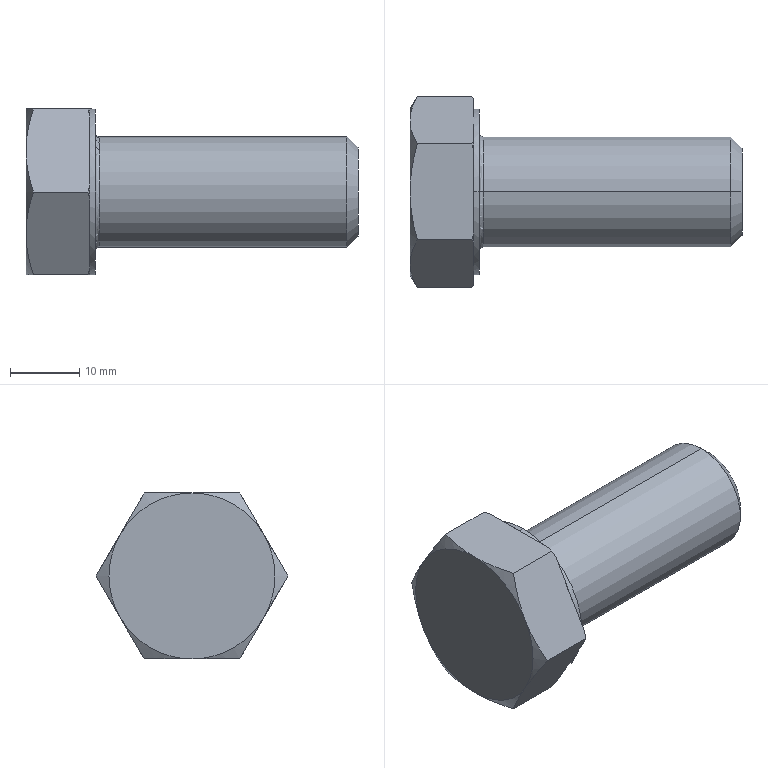Part | SolidWorks | features RevCut 4, Chamfer 1, Extrusion 1, Fillet 1, LPattern 1, Revolution 1 | 1 solid | 35 faces | box 48 x 27.713 x 24 mm | volume 12520 mm3 | plane 15 | cone 14 | cylinder 4 | torus 2 | commonest cylinder face diameters 16 x2 24 x2
STEP:
#1=CARTESIAN_POINT('',(10.6,0.,8.));
#2=VERTEX_POINT('',#1);
#3=CARTESIAN_POINT('',(10.6,0.,-8.));
#4=VERTEX_POINT('',#3);
#5=CARTESIAN_POINT('',(10.6,0.,0.));
#6=DIRECTION('',(1.,0.,0.));
#7=DIRECTION('',(0.,0.,-1.));
#8=AXIS2_PLACEMENT_3D('',#5,#6,#7);
#9=CIRCLE('',#8,8.);
#10=EDGE_CURVE('',#2,#4,#9,.T.);
#11=ORIENTED_EDGE('',*,*,#10,.F.);
#12=CARTESIAN_POINT('',(10.,0.,8.6));
#13=VERTEX_POINT('',#12);
#14=CARTESIAN_POINT('',(10.6,0.,8.6));
#15=DIRECTION('',(0.,1.,0.));
#16=DIRECTION('',(0.,0.,1.));
#17=AXIS2_PLACEMENT_3D('',#14,#15,#16);
#18=CIRCLE('',#17,0.6);
#19=EDGE_CURVE('',#2,#13,#18,.T.);
#20=ORIENTED_EDGE('',*,*,#19,.T.);
#21=CARTESIAN_POINT('',(10.,0.,-8.6));
#22=VERTEX_POINT('',#21);
#23=CARTESIAN_POINT('',(10.,0.,0.));
#24=DIRECTION('',(-1.,0.,0.));
#25=DIRECTION('',(0.,0.,-1.));
#26=AXIS2_PLACEMENT_3D('',#23,#24,#25);
#27=CIRCLE('',#26,8.6);
#28=EDGE_CURVE('',#22,#13,#27,.T.);
#29=ORIENTED_EDGE('',*,*,#28,.F.);
#30=CARTESIAN_POINT('',(10.6,0.,-8.6));
#31=DIRECTION('',(0.,-1.,0.));
#32=DIRECTION('',(0.,0.,-1.));
#33=AXIS2_PLACEMENT_3D('',#30,#31,#32);
#34=CIRCLE('',#33,0.6);
#35=EDGE_CURVE('',#4,#22,#34,.T.);
#36=ORIENTED_EDGE('',*,*,#35,.F.);
#37=EDGE_LOOP('',(#11,#20,#29,#36));
#38=FACE_OUTER_BOUND('',#37,.T.);
#39=CARTESIAN_POINT('',(10.6,0.,0.));
#40=DIRECTION('',(1.,0.,0.));
#41=DIRECTION('',(0.,0.,-1.));
#42=AXIS2_PLACEMENT_3D('',#39,#40,#41);
#43=TOROIDAL_SURFACE('',#42,8.6,0.6);
#44=ADVANCED_FACE('',(#38),#43,.F.);
#45=CARTESIAN_POINT('',(48.,0.,-6.4));
#46=VERTEX_POINT('',#45);
#47=CARTESIAN_POINT('',(48.,0.,6.4));
#48=VERTEX_POINT('',#47);
#49=CARTESIAN_POINT('',(48.,0.,0.));
#50=DIRECTION('',(1.,0.,0.));
#51=DIRECTION('',(0.,0.,1.));
#52=AXIS2_PLACEMENT_3D('',#49,#50,#51);
#53=CIRCLE('',#52,6.4);
#54=EDGE_CURVE('',#46,#48,#53,.T.);
#55=ORIENTED_EDGE('',*,*,#54,.F.);
#56=CARTESIAN_POINT('',(46.4,0.,-8.));
#57=VERTEX_POINT('',#56);
#58=CARTESIAN_POINT('',(46.4,0.,-8.));
#59=DIRECTION('',(-0.7071,0.,-0.7071));
#60=VECTOR('',#59,1000.);
#61=LINE('',#58,#60);
#62=EDGE_CURVE('',#46,#57,#61,.T.);
#63=ORIENTED_EDGE('',*,*,#62,.T.);
#64=CARTESIAN_POINT('',(46.4,0.,8.));
#65=VERTEX_POINT('',#64);
#66=CARTESIAN_POINT('',(46.4,0.,0.));
#67=DIRECTION('',(-1.,0.,0.));
#68=DIRECTION('',(0.,0.,1.));
#69=AXIS2_PLACEMENT_3D('',#66,#67,#68);
#70=CIRCLE('',#69,8.);
#71=EDGE_CURVE('',#65,#57,#70,.T.);
#72=ORIENTED_EDGE('',*,*,#71,.F.);
#73=CARTESIAN_POINT('',(46.4,0.,8.));
#74=DIRECTION('',(-0.7071,0.,0.7071));
#75=VECTOR('',#74,1000.);
#76=LINE('',#73,#75);
#77=EDGE_CURVE('',#48,#65,#76,.T.);
#78=ORIENTED_EDGE('',*,*,#77,.F.);
#79=EDGE_LOOP('',(#55,#63,#72,#78));
#80=FACE_OUTER_BOUND('',#79,.T.);
#81=CARTESIAN_POINT('',(46.4,0.,0.));
#82=DIRECTION('',(-1.,0.,0.));
#83=DIRECTION('',(0.,0.,1.));
#84=AXIS2_PLACEMENT_3D('',#81,#82,#83);
#85=CONICAL_SURFACE('',#84,8.,0.7854);
#86=ADVANCED_FACE('',(#80),#85,.T.);
#87=ORIENTED_EDGE('',*,*,#71,.T.);
#88=CARTESIAN_POINT('',(0.,0.,-8.));
#89=DIRECTION('',(-1.,0.,0.));
#90=VECTOR('',#89,1000.);
#91=LINE('',#88,#90);
#92=EDGE_CURVE('',#57,#4,#91,.T.);
#93=ORIENTED_EDGE('',*,*,#92,.T.);
#94=CARTESIAN_POINT('',(10.6,0.,0.));
#95=DIRECTION('',(1.,0.,0.));
#96=DIRECTION('',(0.,0.,-1.));
#97=AXIS2_PLACEMENT_3D('',#94,#95,#96);
#98=CIRCLE('',#97,8.);
#99=EDGE_CURVE('',#4,#2,#98,.T.);
#100=ORIENTED_EDGE('',*,*,#99,.T.);
#101=CARTESIAN_POINT('',(0.,0.,8.));
#102=DIRECTION('',(-1.,0.,0.));
#103=VECTOR('',#102,1000.);
#104=LINE('',#101,#103);
#105=EDGE_CURVE('',#65,#2,#104,.T.);
#106=ORIENTED_EDGE('',*,*,#105,.F.);
#107=EDGE_LOOP('',(#87,#93,#100,#106));
#108=FACE_OUTER_BOUND('',#107,.T.);
#109=CARTESIAN_POINT('',(0.,0.,0.));
#110=DIRECTION('',(-1.,0.,0.));
#111=DIRECTION('',(0.,0.,1.));
#112=AXIS2_PLACEMENT_3D('',#109,#110,#111);
#113=CYLINDRICAL_SURFACE('',#112,8.);
#114=ADVANCED_FACE('',(#108),#113,.T.);
#115=CARTESIAN_POINT('',(10.,0.,-12.));
#116=VERTEX_POINT('',#115);
#117=CARTESIAN_POINT('',(10.,0.,12.));
#118=VERTEX_POINT('',#117);
#119=CARTESIAN_POINT('',(10.,0.,0.));
#120=DIRECTION('',(1.,0.,0.));
#121=DIRECTION('',(0.,0.,-1.));
#122=AXIS2_PLACEMENT_3D('',#119,#120,#121);
#123=CIRCLE('',#122,12.);
#124=EDGE_CURVE('',#116,#118,#123,.T.);
#125=ORIENTED_EDGE('',*,*,#124,.F.);
#126=CARTESIAN_POINT('',(9.2,0.,-12.));
#127=VERTEX_POINT('',#126);
#128=CARTESIAN_POINT('',(0.,0.,-12.));
#129=DIRECTION('',(-1.,0.,0.));
#130=VECTOR('',#129,1000.);
#131=LINE('',#128,#130);
#132=EDGE_CURVE('',#116,#127,#131,.T.);
#133=ORIENTED_EDGE('',*,*,#132,.T.);
#134=CARTESIAN_POINT('',(9.2,10.392,-6.));
#135=VERTEX_POINT('',#134);
#136=CARTESIAN_POINT('',(9.2,0.,0.));
#137=DIRECTION('',(-1.,0.,0.));
#138=DIRECTION('',(0.,0.,1.));
#139=AXIS2_PLACEMENT_3D('',#136,#137,#138);
#140=CIRCLE('',#139,12.);
#141=EDGE_CURVE('',#135,#127,#140,.T.);
#142=ORIENTED_EDGE('',*,*,#141,.F.);
#143=CARTESIAN_POINT('',(9.2,10.392,6.));
#144=VERTEX_POINT('',#143);
#145=CARTESIAN_POINT('',(9.2,0.,0.));
#146=DIRECTION('',(-1.,0.,0.));
#147=DIRECTION('',(0.,0.,1.));
#148=AXIS2_PLACEMENT_3D('',#145,#146,#147);
#149=CIRCLE('',#148,12.);
#150=EDGE_CURVE('',#144,#135,#149,.T.);
#151=ORIENTED_EDGE('',*,*,#150,.F.);
#152=CARTESIAN_POINT('',(9.2,0.,12.));
#153=VERTEX_POINT('',#152);
#154=CARTESIAN_POINT('',(9.2,0.,0.));
#155=DIRECTION('',(-1.,0.,0.));
#156=DIRECTION('',(0.,0.,1.));
#157=AXIS2_PLACEMENT_3D('',#154,#155,#156);
#158=CIRCLE('',#157,12.);
#159=EDGE_CURVE('',#153,#144,#158,.T.);
#160=ORIENTED_EDGE('',*,*,#159,.F.);
#161=CARTESIAN_POINT('',(0.,0.,12.));
#162=DIRECTION('',(-1.,0.,0.));
#163=VECTOR('',#162,1000.);
#164=LINE('',#161,#163);
#165=EDGE_CURVE('',#118,#153,#164,.T.);
#166=ORIENTED_EDGE('',*,*,#165,.F.);
#167=EDGE_LOOP('',(#125,#133,#142,#151,#160,#166));
#168=FACE_OUTER_BOUND('',#167,.T.);
#169=CARTESIAN_POINT('',(0.,0.,0.));
#170=DIRECTION('',(-1.,0.,0.));
#171=DIRECTION('',(0.,0.,1.));
#172=AXIS2_PLACEMENT_3D('',#169,#170,#171);
#173=CYLINDRICAL_SURFACE('',#172,12.);
#174=ADVANCED_FACE('',(#168),#173,.T.);
#175=CARTESIAN_POINT('',(9.2,7.427,-11.136));
#176=VERTEX_POINT('',#175);
#177=CARTESIAN_POINT('',(9.2,6.928,-12.));
#178=DIRECTION('',(0.,0.5,0.866));
#179=VECTOR('',#178,1000.);
#180=LINE('',#177,#179);
#181=EDGE_CURVE('',#176,#135,#180,.T.);
#182=ORIENTED_EDGE('',*,*,#181,.F.);
#183=CARTESIAN_POINT('',(8.928,6.928,-12.));
#184=VERTEX_POINT('',#183);
#185=CARTESIAN_POINT('',(8.928,6.928,-12.));
#186=CARTESIAN_POINT('',(9.024,7.094,-11.713));
#187=CARTESIAN_POINT('',(9.115,7.26,-11.425));
#188=CARTESIAN_POINT('',(9.2,7.427,-11.136));
#189=B_SPLINE_CURVE_WITH_KNOTS('',3,(#185,#186,#187,#188),.UNSPECIFIED.,.F.,.F.,(4,4),(0.000000238,0.001026),.UNSPECIFIED.);
#190=EDGE_CURVE('',#184,#176,#189,.T.);
#191=ORIENTED_EDGE('',*,*,#190,.F.);
#192=CARTESIAN_POINT('',(1.072,6.928,-12.));
#193=VERTEX_POINT('',#192);
#194=CARTESIAN_POINT('',(10.,6.928,-12.));
#195=DIRECTION('',(-1.,0.,0.));
#196=VECTOR('',#195,1000.);
#197=LINE('',#194,#196);
#198=EDGE_CURVE('',#184,#193,#197,.T.);
#199=ORIENTED_EDGE('',*,*,#198,.T.);
#200=CARTESIAN_POINT('',(0.,10.392,-6.));
#201=VERTEX_POINT('',#200);
#202=CARTESIAN_POINT('',(0.,10.392,-6.));
#203=CARTESIAN_POINT('',(0.,10.098,-6.509));
#204=CARTESIAN_POINT('',(0.02533,9.803,-7.021));
#205=CARTESIAN_POINT('',(0.1234,9.219,-8.033));
#206=CARTESIAN_POINT('',(0.196,8.929,-8.535));
#207=CARTESIAN_POINT('',(0.476,8.063,-10.034));
#208=CARTESIAN_POINT('',(0.7454,7.493,-11.021));
#209=CARTESIAN_POINT('',(1.072,6.928,-12.));
#210=B_SPLINE_CURVE_WITH_KNOTS('',3,(#202,#203,#204,#205,#206,#207,#208,#209),.UNSPECIFIED.,.F.,.F.,(4,2,2,4),(0.00701,0.008756,0.0105,0.01399),.UNSPECIFIED.);
#211=EDGE_CURVE('',#201,#193,#210,.T.);
#212=ORIENTED_EDGE('',*,*,#211,.F.);
#213=CARTESIAN_POINT('',(1.072,13.856,0.));
#214=VERTEX_POINT('',#213);
#215=CARTESIAN_POINT('',(1.072,13.856,0.));
#216=CARTESIAN_POINT('',(0.7446,13.29,-0.9815));
#217=CARTESIAN_POINT('',(0.4751,12.719,-1.97));
#218=CARTESIAN_POINT('',(0.1021,11.565,-3.968));
#219=CARTESIAN_POINT('',(0.,10.982,-4.978));
#220=CARTESIAN_POINT('',(0.,10.392,-6.));
#221=B_SPLINE_CURVE_WITH_KNOTS('',3,(#215,#216,#217,#218,#219,#220),.UNSPECIFIED.,.F.,.F.,(4,2,4),(0.000000238,0.003505,0.00701),.UNSPECIFIED.);
#222=EDGE_CURVE('',#214,#201,#221,.T.);
#223=ORIENTED_EDGE('',*,*,#222,.F.);
#224=CARTESIAN_POINT('',(8.928,13.856,0.));
#225=VERTEX_POINT('',#224);
#226=CARTESIAN_POINT('',(10.,13.856,0.));
#227=DIRECTION('',(-1.,0.,0.));
#228=VECTOR('',#227,1000.);
#229=LINE('',#226,#228);
#230=EDGE_CURVE('',#225,#214,#229,.T.);
#231=ORIENTED_EDGE('',*,*,#230,.F.);
#232=CARTESIAN_POINT('',(9.2,13.358,-0.8637));
#233=VERTEX_POINT('',#232);
#234=CARTESIAN_POINT('',(9.2,13.358,-0.8637));
#235=CARTESIAN_POINT('',(9.115,13.524,-0.575));
#236=CARTESIAN_POINT('',(9.024,13.691,-0.2872));
#237=CARTESIAN_POINT('',(8.928,13.856,0.));
#238=B_SPLINE_CURVE_WITH_KNOTS('',3,(#234,#235,#236,#237),.UNSPECIFIED.,.F.,.F.,(4,4),(0.01297,0.01399),.UNSPECIFIED.);
#239=EDGE_CURVE('',#233,#225,#238,.T.);
#240=ORIENTED_EDGE('',*,*,#239,.F.);
#241=CARTESIAN_POINT('',(9.2,6.928,-12.));
#242=DIRECTION('',(0.,0.5,0.866));
#243=VECTOR('',#242,1000.);
#244=LINE('',#241,#243);
#245=EDGE_CURVE('',#135,#233,#244,.T.);
#246=ORIENTED_EDGE('',*,*,#245,.F.);
#247=EDGE_LOOP('',(#182,#191,#199,#212,#223,#231,#240,#246));
#248=FACE_OUTER_BOUND('',#247,.T.);
#249=CARTESIAN_POINT('',(10.,6.928,-12.));
#250=DIRECTION('',(0.,-0.866,0.5));
#251=DIRECTION('',(0.,-0.5,-0.866));
#252=AXIS2_PLACEMENT_3D('',#249,#250,#251);
#253=PLANE('',#252);
#254=ADVANCED_FACE('',(#248),#253,.F.);
#255=CARTESIAN_POINT('',(9.2,13.358,0.8637));
#256=VERTEX_POINT('',#255);
#257=CARTESIAN_POINT('',(9.2,13.856,0.));
#258=DIRECTION('',(0.,-0.5,0.866));
#259=VECTOR('',#258,1000.);
#260=LINE('',#257,#259);
#261=EDGE_CURVE('',#256,#144,#260,.T.);
#262=ORIENTED_EDGE('',*,*,#261,.F.);
#263=CARTESIAN_POINT('',(8.928,13.856,0.));
#264=CARTESIAN_POINT('',(9.024,13.691,0.2873));
#265=CARTESIAN_POINT('',(9.115,13.524,0.5751));
#266=CARTESIAN_POINT('',(9.2,13.358,0.8637));
#267=B_SPLINE_CURVE_WITH_KNOTS('',3,(#263,#264,#265,#266),.UNSPECIFIED.,.F.,.F.,(4,4),(0.000000238,0.001026),.UNSPECIFIED.);
#268=EDGE_CURVE('',#225,#256,#267,.T.);
#269=ORIENTED_EDGE('',*,*,#268,.F.);
#270=ORIENTED_EDGE('',*,*,#230,.T.);
#271=CARTESIAN_POINT('',(0.,10.392,6.));
#272=VERTEX_POINT('',#271);
#273=CARTESIAN_POINT('',(0.,10.392,6.));
#274=CARTESIAN_POINT('',(0.,10.686,5.491));
#275=CARTESIAN_POINT('',(0.02533,10.982,4.979));
#276=CARTESIAN_POINT('',(0.1234,11.566,3.967));
#277=CARTESIAN_POINT('',(0.196,11.856,3.465));
#278=CARTESIAN_POINT('',(0.476,12.721,1.966));
#279=CARTESIAN_POINT('',(0.7454,13.291,0.9791));
#280=CARTESIAN_POINT('',(1.072,13.856,0.));
#281=B_SPLINE_CURVE_WITH_KNOTS('',3,(#273,#274,#275,#276,#277,#278,#279,#280),.UNSPECIFIED.,.F.,.F.,(4,2,2,4),(0.00701,0.008756,0.0105,0.01399),.UNSPECIFIED.);
#282=EDGE_CURVE('',#272,#214,#281,.T.);
#283=ORIENTED_EDGE('',*,*,#282,.F.);
#284=CARTESIAN_POINT('',(1.072,6.928,12.));
#285=VERTEX_POINT('',#284);
#286=CARTESIAN_POINT('',(1.072,6.928,12.));
#287=CARTESIAN_POINT('',(0.7446,7.495,11.018));
#288=CARTESIAN_POINT('',(0.4751,8.066,10.03));
#289=CARTESIAN_POINT('',(0.1021,9.219,8.032));
#290=CARTESIAN_POINT('',(0.,9.802,7.022));
#291=CARTESIAN_POINT('',(0.,10.392,6.));
#292=B_SPLINE_CURVE_WITH_KNOTS('',3,(#286,#287,#288,#289,#290,#291),.UNSPECIFIED.,.F.,.F.,(4,2,4),(0.000000238,0.003505,0.00701),.UNSPECIFIED.);
#293=EDGE_CURVE('',#285,#272,#292,.T.);
#294=ORIENTED_EDGE('',*,*,#293,.F.);
#295=CARTESIAN_POINT('',(8.928,6.928,12.));
#296=VERTEX_POINT('',#295);
#297=CARTESIAN_POINT('',(10.,6.928,12.));
#298=DIRECTION('',(-1.,0.,0.));
#299=VECTOR('',#298,1000.);
#300=LINE('',#297,#299);
#301=EDGE_CURVE('',#296,#285,#300,.T.);
#302=ORIENTED_EDGE('',*,*,#301,.F.);
#303=CARTESIAN_POINT('',(9.2,7.427,11.136));
#304=VERTEX_POINT('',#303);
#305=CARTESIAN_POINT('',(9.2,7.427,11.136));
#306=CARTESIAN_POINT('',(9.115,7.26,11.425));
#307=CARTESIAN_POINT('',(9.024,7.094,11.713));
#308=CARTESIAN_POINT('',(8.928,6.928,12.));
#309=B_SPLINE_CURVE_WITH_KNOTS('',3,(#305,#306,#307,#308),.UNSPECIFIED.,.F.,.F.,(4,4),(0.01297,0.01399),.UNSPECIFIED.);
#310=EDGE_CURVE('',#304,#296,#309,.T.);
#311=ORIENTED_EDGE('',*,*,#310,.F.);
#312=CARTESIAN_POINT('',(9.2,13.856,0.));
#313=DIRECTION('',(0.,-0.5,0.866));
#314=VECTOR('',#313,1000.);
#315=LINE('',#312,#314);
#316=EDGE_CURVE('',#144,#304,#315,.T.);
#317=ORIENTED_EDGE('',*,*,#316,.F.);
#318=EDGE_LOOP('',(#262,#269,#270,#283,#294,#302,#311,#317));
#319=FACE_OUTER_BOUND('',#318,.T.);
#320=CARTESIAN_POINT('',(10.,13.856,0.));
#321=DIRECTION('',(0.,-0.866,-0.5));
#322=DIRECTION('',(0.,0.5,-0.866));
#323=AXIS2_PLACEMENT_3D('',#320,#321,#322);
#324=PLANE('',#323);
#325=ADVANCED_FACE('',(#319),#324,.F.);
#326=CARTESIAN_POINT('',(9.2,5.931,12.));
#327=VERTEX_POINT('',#326);
#328=CARTESIAN_POINT('',(9.2,6.928,12.));
#329=DIRECTION('',(0.,-1.,0.));
#330=VECTOR('',#329,1000.);
#331=LINE('',#328,#330);
#332=EDGE_CURVE('',#327,#153,#331,.T.);
#333=ORIENTED_EDGE('',*,*,#332,.F.);
#334=CARTESIAN_POINT('',(8.928,6.928,12.));
#335=CARTESIAN_POINT('',(9.024,6.597,12.));
#336=CARTESIAN_POINT('',(9.115,6.265,12.));
#337=CARTESIAN_POINT('',(9.2,5.931,12.));
#338=B_SPLINE_CURVE_WITH_KNOTS('',3,(#334,#335,#336,#337),.UNSPECIFIED.,.F.,.F.,(4,4),(0.03236,0.0334),.UNSPECIFIED.);
#339=EDGE_CURVE('',#296,#327,#338,.T.);
#340=ORIENTED_EDGE('',*,*,#339,.F.);
#341=ORIENTED_EDGE('',*,*,#301,.T.);
#342=CARTESIAN_POINT('',(0.,0.,12.));
#343=VERTEX_POINT('',#342);
#344=CARTESIAN_POINT('',(0.,0.,12.));
#345=CARTESIAN_POINT('',(0.,0.5865,12.));
#346=CARTESIAN_POINT('',(0.02506,1.176,12.));
#347=CARTESIAN_POINT('',(0.1242,2.355,12.));
#348=CARTESIAN_POINT('',(0.1975,2.939,12.));
#349=CARTESIAN_POINT('',(0.4791,4.673,12.));
#350=CARTESIAN_POINT('',(0.7483,5.808,12.));
#351=CARTESIAN_POINT('',(1.072,6.928,12.));
#352=B_SPLINE_CURVE_WITH_KNOTS('',3,(#344,#345,#346,#347,#348,#349,#350,#351),.UNSPECIFIED.,.F.,.F.,(4,2,2,4),(0.01982,0.02158,0.02333,0.02684),.UNSPECIFIED.);
#353=EDGE_CURVE('',#343,#285,#352,.T.);
#354=ORIENTED_EDGE('',*,*,#353,.F.);
#355=CARTESIAN_POINT('',(1.072,-6.928,12.));
#356=VERTEX_POINT('',#355);
#357=CARTESIAN_POINT('',(1.072,-6.928,12.));
#358=CARTESIAN_POINT('',(0.7461,-5.8,12.));
#359=CARTESIAN_POINT('',(0.4736,-4.647,12.));
#360=CARTESIAN_POINT('',(0.1008,-2.335,12.));
#361=CARTESIAN_POINT('',(0.,-1.172,12.));
#362=CARTESIAN_POINT('',(0.,0.,12.));
#363=B_SPLINE_CURVE_WITH_KNOTS('',3,(#357,#358,#359,#360,#361,#362),.UNSPECIFIED.,.F.,.F.,(4,2,4),(0.01281,0.01632,0.01982),.UNSPECIFIED.);
#364=EDGE_CURVE('',#356,#343,#363,.T.);
#365=ORIENTED_EDGE('',*,*,#364,.F.);
#366=CARTESIAN_POINT('',(8.928,-6.928,12.));
#367=VERTEX_POINT('',#366);
#368=CARTESIAN_POINT('',(10.,-6.928,12.));
#369=DIRECTION('',(-1.,0.,0.));
#370=VECTOR('',#369,1000.);
#371=LINE('',#368,#370);
#372=EDGE_CURVE('',#367,#356,#371,.T.);
#373=ORIENTED_EDGE('',*,*,#372,.F.);
#374=CARTESIAN_POINT('',(9.2,-5.931,12.));
#375=VERTEX_POINT('',#374);
#376=CARTESIAN_POINT('',(9.2,-5.931,12.));
#377=CARTESIAN_POINT('',(9.114,-6.265,12.));
#378=CARTESIAN_POINT('',(9.024,-6.598,12.));
#379=CARTESIAN_POINT('',(8.928,-6.928,12.));
#380=B_SPLINE_CURVE_WITH_KNOTS('',3,(#376,#377,#378,#379),.UNSPECIFIED.,.F.,.F.,(4,4),(0.04537,0.0464),.UNSPECIFIED.);
#381=EDGE_CURVE('',#375,#367,#380,.T.);
#382=ORIENTED_EDGE('',*,*,#381,.F.);
#383=CARTESIAN_POINT('',(9.2,6.928,12.));
#384=DIRECTION('',(0.,-1.,0.));
#385=VECTOR('',#384,1000.);
#386=LINE('',#383,#385);
#387=EDGE_CURVE('',#153,#375,#386,.T.);
#388=ORIENTED_EDGE('',*,*,#387,.F.);
#389=EDGE_LOOP('',(#333,#340,#341,#354,#365,#373,#382,#388));
#390=FACE_OUTER_BOUND('',#389,.T.);
#391=CARTESIAN_POINT('',(10.,6.928,12.));
#392=DIRECTION('',(0.,0.,-1.));
#393=DIRECTION('',(-1.,0.,0.));
#394=AXIS2_PLACEMENT_3D('',#391,#392,#393);
#395=PLANE('',#394);
#396=ADVANCED_FACE('',(#390),#395,.F.);
#397=CARTESIAN_POINT('',(9.2,-7.427,11.136));
#398=VERTEX_POINT('',#397);
#399=CARTESIAN_POINT('',(9.2,-10.392,6.));
#400=VERTEX_POINT('',#399);
#401=CARTESIAN_POINT('',(9.2,-13.856,0.));
#402=DIRECTION('',(0.,-0.5,-0.866));
#403=VECTOR('',#402,1000.);
#404=LINE('',#401,#403);
#405=EDGE_CURVE('',#398,#400,#404,.T.);
#406=ORIENTED_EDGE('',*,*,#405,.F.);
#407=CARTESIAN_POINT('',(8.928,-6.928,12.));
#408=CARTESIAN_POINT('',(9.024,-7.094,11.713));
#409=CARTESIAN_POINT('',(9.115,-7.26,11.425));
#410=CARTESIAN_POINT('',(9.2,-7.427,11.136));
#411=B_SPLINE_CURVE_WITH_KNOTS('',3,(#407,#408,#409,#410),.UNSPECIFIED.,.F.,.F.,(4,4),(0.000000238,0.001026),.UNSPECIFIED.);
#412=EDGE_CURVE('',#367,#398,#411,.T.);
#413=ORIENTED_EDGE('',*,*,#412,.F.);
#414=ORIENTED_EDGE('',*,*,#372,.T.);
#415=CARTESIAN_POINT('',(0.,-10.392,6.));
#416=VERTEX_POINT('',#415);
#417=CARTESIAN_POINT('',(0.,-10.392,6.));
#418=CARTESIAN_POINT('',(0.,-10.098,6.509));
#419=CARTESIAN_POINT('',(0.02533,-9.803,7.021));
#420=CARTESIAN_POINT('',(0.1234,-9.219,8.033));
#421=CARTESIAN_POINT('',(0.196,-8.929,8.535));
#422=CARTESIAN_POINT('',(0.476,-8.063,10.034));
#423=CARTESIAN_POINT('',(0.7454,-7.493,11.021));
#424=CARTESIAN_POINT('',(1.072,-6.928,12.));
#425=B_SPLINE_CURVE_WITH_KNOTS('',3,(#417,#418,#419,#420,#421,#422,#423,#424),.UNSPECIFIED.,.F.,.F.,(4,2,2,4),(0.00701,0.008756,0.0105,0.01399),.UNSPECIFIED.);
#426=EDGE_CURVE('',#416,#356,#425,.T.);
#427=ORIENTED_EDGE('',*,*,#426,.F.);
#428=CARTESIAN_POINT('',(1.072,-13.856,0.));
#429=VERTEX_POINT('',#428);
#430=CARTESIAN_POINT('',(1.072,-13.856,0.));
#431=CARTESIAN_POINT('',(0.7446,-13.29,0.9815));
#432=CARTESIAN_POINT('',(0.4751,-12.719,1.97));
#433=CARTESIAN_POINT('',(0.1021,-11.565,3.968));
#434=CARTESIAN_POINT('',(0.,-10.982,4.978));
#435=CARTESIAN_POINT('',(0.,-10.392,6.));
#436=B_SPLINE_CURVE_WITH_KNOTS('',3,(#430,#431,#432,#433,#434,#435),.UNSPECIFIED.,.F.,.F.,(4,2,4),(0.000000238,0.003505,0.00701),.UNSPECIFIED.);
#437=EDGE_CURVE('',#429,#416,#436,.T.);
#438=ORIENTED_EDGE('',*,*,#437,.F.);
#439=CARTESIAN_POINT('',(8.928,-13.856,0.));
#440=VERTEX_POINT('',#439);
#441=CARTESIAN_POINT('',(10.,-13.856,0.));
#442=DIRECTION('',(-1.,0.,0.));
#443=VECTOR('',#442,1000.);
#444=LINE('',#441,#443);
#445=EDGE_CURVE('',#440,#429,#444,.T.);
#446=ORIENTED_EDGE('',*,*,#445,.F.);
#447=CARTESIAN_POINT('',(9.2,-13.358,0.8637));
#448=VERTEX_POINT('',#447);
#449=CARTESIAN_POINT('',(9.2,-13.358,0.8637));
#450=CARTESIAN_POINT('',(9.115,-13.524,0.575));
#451=CARTESIAN_POINT('',(9.024,-13.691,0.2872));
#452=CARTESIAN_POINT('',(8.928,-13.856,0.));
#453=B_SPLINE_CURVE_WITH_KNOTS('',3,(#449,#450,#451,#452),.UNSPECIFIED.,.F.,.F.,(4,4),(0.01297,0.01399),.UNSPECIFIED.);
#454=EDGE_CURVE('',#448,#440,#453,.T.);
#455=ORIENTED_EDGE('',*,*,#454,.F.);
#456=CARTESIAN_POINT('',(9.2,-13.856,0.));
#457=DIRECTION('',(0.,-0.5,-0.866));
#458=VECTOR('',#457,1000.);
#459=LINE('',#456,#458);
#460=EDGE_CURVE('',#400,#448,#459,.T.);
#461=ORIENTED_EDGE('',*,*,#460,.F.);
#462=EDGE_LOOP('',(#406,#413,#414,#427,#438,#446,#455,#461));
#463=FACE_OUTER_BOUND('',#462,.T.);
#464=CARTESIAN_POINT('',(10.,-13.856,0.));
#465=DIRECTION('',(0.,0.866,-0.5));
#466=DIRECTION('',(0.,0.5,0.866));
#467=AXIS2_PLACEMENT_3D('',#464,#465,#466);
#468=PLANE('',#467);
#469=ADVANCED_FACE('',(#463),#468,.F.);
#470=CARTESIAN_POINT('',(9.2,-13.358,-0.8637));
#471=VERTEX_POINT('',#470);
#472=CARTESIAN_POINT('',(9.2,-10.392,-6.));
#473=VERTEX_POINT('',#472);
#474=CARTESIAN_POINT('',(9.2,-6.928,-12.));
#475=DIRECTION('',(0.,0.5,-0.866));
#476=VECTOR('',#475,1000.);
#477=LINE('',#474,#476);
#478=EDGE_CURVE('',#471,#473,#477,.T.);
#479=ORIENTED_EDGE('',*,*,#478,.F.);
#480=CARTESIAN_POINT('',(8.928,-13.856,0.));
#481=CARTESIAN_POINT('',(9.024,-13.691,-0.2873));
#482=CARTESIAN_POINT('',(9.115,-13.524,-0.5751));
#483=CARTESIAN_POINT('',(9.2,-13.358,-0.8637));
#484=B_SPLINE_CURVE_WITH_KNOTS('',3,(#480,#481,#482,#483),.UNSPECIFIED.,.F.,.F.,(4,4),(0.000000238,0.001026),.UNSPECIFIED.);
#485=EDGE_CURVE('',#440,#471,#484,.T.);
#486=ORIENTED_EDGE('',*,*,#485,.F.);
#487=ORIENTED_EDGE('',*,*,#445,.T.);
#488=CARTESIAN_POINT('',(0.,-10.392,-6.));
#489=VERTEX_POINT('',#488);
#490=CARTESIAN_POINT('',(0.,-10.392,-6.));
#491=CARTESIAN_POINT('',(0.,-10.686,-5.491));
#492=CARTESIAN_POINT('',(0.02533,-10.982,-4.979));
#493=CARTESIAN_POINT('',(0.1234,-11.566,-3.967));
#494=CARTESIAN_POINT('',(0.196,-11.856,-3.465));
#495=CARTESIAN_POINT('',(0.476,-12.721,-1.966));
#496=CARTESIAN_POINT('',(0.7454,-13.291,-0.9791));
#497=CARTESIAN_POINT('',(1.072,-13.856,0.));
#498=B_SPLINE_CURVE_WITH_KNOTS('',3,(#490,#491,#492,#493,#494,#495,#496,#497),.UNSPECIFIED.,.F.,.F.,(4,2,2,4),(0.00701,0.008756,0.0105,0.01399),.UNSPECIFIED.);
#499=EDGE_CURVE('',#489,#429,#498,.T.);
#500=ORIENTED_EDGE('',*,*,#499,.F.);
#501=CARTESIAN_POINT('',(1.072,-6.928,-12.));
#502=VERTEX_POINT('',#501);
#503=CARTESIAN_POINT('',(1.072,-6.928,-12.));
#504=CARTESIAN_POINT('',(0.7446,-7.495,-11.018));
#505=CARTESIAN_POINT('',(0.4751,-8.066,-10.03));
#506=CARTESIAN_POINT('',(0.1021,-9.219,-8.032));
#507=CARTESIAN_POINT('',(0.,-9.802,-7.022));
#508=CARTESIAN_POINT('',(0.,-10.392,-6.));
#509=B_SPLINE_CURVE_WITH_KNOTS('',3,(#503,#504,#505,#506,#507,#508),.UNSPECIFIED.,.F.,.F.,(4,2,4),(0.000000238,0.003505,0.00701),.UNSPECIFIED.);
#510=EDGE_CURVE('',#502,#489,#509,.T.);
#511=ORIENTED_EDGE('',*,*,#510,.F.);
#512=CARTESIAN_POINT('',(8.928,-6.928,-12.));
#513=VERTEX_POINT('',#512);
#514=CARTESIAN_POINT('',(10.,-6.928,-12.));
#515=DIRECTION('',(-1.,0.,0.));
#516=VECTOR('',#515,1000.);
#517=LINE('',#514,#516);
#518=EDGE_CURVE('',#513,#502,#517,.T.);
#519=ORIENTED_EDGE('',*,*,#518,.F.);
#520=CARTESIAN_POINT('',(9.2,-7.427,-11.136));
#521=VERTEX_POINT('',#520);
#522=CARTESIAN_POINT('',(9.2,-7.427,-11.136));
#523=CARTESIAN_POINT('',(9.115,-7.26,-11.425));
#524=CARTESIAN_POINT('',(9.024,-7.094,-11.713));
#525=CARTESIAN_POINT('',(8.928,-6.928,-12.));
#526=B_SPLINE_CURVE_WITH_KNOTS('',3,(#522,#523,#524,#525),.UNSPECIFIED.,.F.,.F.,(4,4),(0.01297,0.01399),.UNSPECIFIED.);
#527=EDGE_CURVE('',#521,#513,#526,.T.);
#528=ORIENTED_EDGE('',*,*,#527,.F.);
#529=CARTESIAN_POINT('',(9.2,-6.928,-12.));
#530=DIRECTION('',(0.,0.5,-0.866));
#531=VECTOR('',#530,1000.);
#532=LINE('',#529,#531);
#533=EDGE_CURVE('',#473,#521,#532,.T.);
#534=ORIENTED_EDGE('',*,*,#533,.F.);
#535=EDGE_LOOP('',(#479,#486,#487,#500,#511,#519,#528,#534));
#536=FACE_OUTER_BOUND('',#535,.T.);
#537=CARTESIAN_POINT('',(10.,-6.928,-12.));
#538=DIRECTION('',(0.,0.866,0.5));
#539=DIRECTION('',(0.,-0.5,0.866));
#540=AXIS2_PLACEMENT_3D('',#537,#538,#539);
#541=PLANE('',#540);
#542=ADVANCED_FACE('',(#536),#541,.F.);
#543=CARTESIAN_POINT('',(9.2,-5.931,-12.));
#544=VERTEX_POINT('',#543);
#545=CARTESIAN_POINT('',(9.2,6.928,-12.));
#546=DIRECTION('',(0.,1.,0.));
#547=VECTOR('',#546,1000.);
#548=LINE('',#545,#547);
#549=EDGE_CURVE('',#544,#127,#548,.T.);
#550=ORIENTED_EDGE('',*,*,#549,.F.);
#551=CARTESIAN_POINT('',(8.928,-6.928,-12.));
#552=CARTESIAN_POINT('',(9.024,-6.598,-12.));
#553=CARTESIAN_POINT('',(9.114,-6.265,-12.));
#554=CARTESIAN_POINT('',(9.2,-5.931,-12.));
#555=B_SPLINE_CURVE_WITH_KNOTS('',3,(#551,#552,#553,#554),.UNSPECIFIED.,.F.,.F.,(4,4),(0.01281,0.01384),.UNSPECIFIED.);
#556=EDGE_CURVE('',#513,#544,#555,.T.);
#557=ORIENTED_EDGE('',*,*,#556,.F.);
#558=ORIENTED_EDGE('',*,*,#518,.T.);
#559=CARTESIAN_POINT('',(0.,0.,-12.));
#560=VERTEX_POINT('',#559);
#561=CARTESIAN_POINT('',(0.,0.,-12.));
#562=CARTESIAN_POINT('',(0.,-1.172,-12.));
#563=CARTESIAN_POINT('',(0.1008,-2.335,-12.));
#564=CARTESIAN_POINT('',(0.4736,-4.647,-12.));
#565=CARTESIAN_POINT('',(0.7461,-5.8,-12.));
#566=CARTESIAN_POINT('',(1.072,-6.928,-12.));
#567=B_SPLINE_CURVE_WITH_KNOTS('',3,(#561,#562,#563,#564,#565,#566),.UNSPECIFIED.,.F.,.F.,(4,2,4),(0.03938,0.04289,0.0464),.UNSPECIFIED.);
#568=EDGE_CURVE('',#560,#502,#567,.T.);
#569=ORIENTED_EDGE('',*,*,#568,.F.);
#570=CARTESIAN_POINT('',(1.072,6.928,-12.));
#571=CARTESIAN_POINT('',(0.7483,5.808,-12.));
#572=CARTESIAN_POINT('',(0.4791,4.673,-12.));
#573=CARTESIAN_POINT('',(0.1975,2.939,-12.));
#574=CARTESIAN_POINT('',(0.1242,2.355,-12.));
#575=CARTESIAN_POINT('',(0.02506,1.176,-12.));
#576=CARTESIAN_POINT('',(0.,0.5865,-12.));
#577=CARTESIAN_POINT('',(0.,0.,-12.));
#578=B_SPLINE_CURVE_WITH_KNOTS('',3,(#570,#571,#572,#573,#574,#575,#576,#577),.UNSPECIFIED.,.F.,.F.,(4,2,2,4),(0.03236,0.03587,0.03763,0.03938),.UNSPECIFIED.);
#579=EDGE_CURVE('',#193,#560,#578,.T.);
#580=ORIENTED_EDGE('',*,*,#579,.F.);
#581=ORIENTED_EDGE('',*,*,#198,.F.);
#582=CARTESIAN_POINT('',(9.2,5.931,-12.));
#583=VERTEX_POINT('',#582);
#584=CARTESIAN_POINT('',(9.2,5.931,-12.));
#585=CARTESIAN_POINT('',(9.115,6.265,-12.));
#586=CARTESIAN_POINT('',(9.024,6.597,-12.));
#587=CARTESIAN_POINT('',(8.928,6.928,-12.));
#588=B_SPLINE_CURVE_WITH_KNOTS('',3,(#584,#585,#586,#587),.UNSPECIFIED.,.F.,.F.,(4,4),(0.0258,0.02684),.UNSPECIFIED.);
#589=EDGE_CURVE('',#583,#184,#588,.T.);
#590=ORIENTED_EDGE('',*,*,#589,.F.);
#591=CARTESIAN_POINT('',(9.2,6.928,-12.));
#592=DIRECTION('',(0.,1.,0.));
#593=VECTOR('',#592,1000.);
#594=LINE('',#591,#593);
#595=EDGE_CURVE('',#127,#583,#594,.T.);
#596=ORIENTED_EDGE('',*,*,#595,.F.);
#597=EDGE_LOOP('',(#550,#557,#558,#569,#580,#581,#590,#596));
#598=FACE_OUTER_BOUND('',#597,.T.);
#599=CARTESIAN_POINT('',(10.,6.928,-12.));
#600=DIRECTION('',(0.,0.,1.));
#601=DIRECTION('',(0.,-1.,0.));
#602=AXIS2_PLACEMENT_3D('',#599,#600,#601);
#603=PLANE('',#602);
#604=ADVANCED_FACE('',(#598),#603,.F.);
#605=ORIENTED_EDGE('',*,*,#556,.T.);
#606=CARTESIAN_POINT('',(9.2,0.,0.));
#607=DIRECTION('',(-1.,0.,0.));
#608=DIRECTION('',(0.,0.,-1.));
#609=AXIS2_PLACEMENT_3D('',#606,#607,#608);
#610=CIRCLE('',#609,13.386);
#611=EDGE_CURVE('',#544,#521,#610,.T.);
#612=ORIENTED_EDGE('',*,*,#611,.T.);
#613=ORIENTED_EDGE('',*,*,#527,.T.);
#614=EDGE_LOOP('',(#605,#612,#613));
#615=FACE_OUTER_BOUND('',#614,.T.);
#616=CARTESIAN_POINT('',(6.041,0.,0.));
#617=DIRECTION('',(-1.,0.,0.));
#618=DIRECTION('',(0.,0.,1.));
#619=AXIS2_PLACEMENT_3D('',#616,#617,#618);
#620=CONICAL_SURFACE('',#619,18.856,1.047);
#621=ADVANCED_FACE('',(#615),#620,.T.);
#622=ORIENTED_EDGE('',*,*,#485,.T.);
#623=CARTESIAN_POINT('',(9.2,0.,0.));
#624=DIRECTION('',(-1.,0.,0.));
#625=DIRECTION('',(0.,0.,-1.));
#626=AXIS2_PLACEMENT_3D('',#623,#624,#625);
#627=CIRCLE('',#626,13.386);
#628=EDGE_CURVE('',#471,#448,#627,.T.);
#629=ORIENTED_EDGE('',*,*,#628,.T.);
#630=ORIENTED_EDGE('',*,*,#454,.T.);
#631=EDGE_LOOP('',(#622,#629,#630));
#632=FACE_OUTER_BOUND('',#631,.T.);
#633=CARTESIAN_POINT('',(6.041,0.,0.));
#634=DIRECTION('',(-1.,0.,0.));
#635=DIRECTION('',(0.,0.,1.));
#636=AXIS2_PLACEMENT_3D('',#633,#634,#635);
#637=CONICAL_SURFACE('',#636,18.856,1.047);
#638=ADVANCED_FACE('',(#632),#637,.T.);
#639=ORIENTED_EDGE('',*,*,#412,.T.);
#640=CARTESIAN_POINT('',(9.2,0.,0.));
#641=DIRECTION('',(-1.,0.,0.));
#642=DIRECTION('',(0.,0.,-1.));
#643=AXIS2_PLACEMENT_3D('',#640,#641,#642);
#644=CIRCLE('',#643,13.386);
#645=EDGE_CURVE('',#398,#375,#644,.T.);
#646=ORIENTED_EDGE('',*,*,#645,.T.);
#647=ORIENTED_EDGE('',*,*,#381,.T.);
#648=EDGE_LOOP('',(#639,#646,#647));
#649=FACE_OUTER_BOUND('',#648,.T.);
#650=CARTESIAN_POINT('',(6.041,0.,0.));
#651=DIRECTION('',(-1.,0.,0.));
#652=DIRECTION('',(0.,0.,1.));
#653=AXIS2_PLACEMENT_3D('',#650,#651,#652);
#654=CONICAL_SURFACE('',#653,18.856,1.047);
#655=ADVANCED_FACE('',(#649),#654,.T.);
#656=ORIENTED_EDGE('',*,*,#339,.T.);
#657=CARTESIAN_POINT('',(9.2,0.,0.));
#658=DIRECTION('',(-1.,0.,0.));
#659=DIRECTION('',(0.,0.,-1.));
#660=AXIS2_PLACEMENT_3D('',#657,#658,#659);
#661=CIRCLE('',#660,13.386);
#662=EDGE_CURVE('',#327,#304,#661,.T.);
#663=ORIENTED_EDGE('',*,*,#662,.T.);
#664=ORIENTED_EDGE('',*,*,#310,.T.);
#665=EDGE_LOOP('',(#656,#663,#664));
#666=FACE_OUTER_BOUND('',#665,.T.);
#667=CARTESIAN_POINT('',(6.041,0.,0.));
#668=DIRECTION('',(-1.,0.,0.));
#669=DIRECTION('',(0.,0.,1.));
#670=AXIS2_PLACEMENT_3D('',#667,#668,#669);
#671=CONICAL_SURFACE('',#670,18.856,1.047);
#672=ADVANCED_FACE('',(#666),#671,.T.);
#673=ORIENTED_EDGE('',*,*,#268,.T.);
#674=CARTESIAN_POINT('',(9.2,0.,0.));
#675=DIRECTION('',(-1.,0.,0.));
#676=DIRECTION('',(0.,0.,-1.));
#677=AXIS2_PLACEMENT_3D('',#674,#675,#676);
#678=CIRCLE('',#677,13.386);
#679=EDGE_CURVE('',#256,#233,#678,.T.);
#680=ORIENTED_EDGE('',*,*,#679,.T.);
#681=ORIENTED_EDGE('',*,*,#239,.T.);
#682=EDGE_LOOP('',(#673,#680,#681));
#683=FACE_OUTER_BOUND('',#682,.T.);
#684=CARTESIAN_POINT('',(6.041,0.,0.));
#685=DIRECTION('',(-1.,0.,0.));
#686=DIRECTION('',(0.,0.,1.));
#687=AXIS2_PLACEMENT_3D('',#684,#685,#686);
#688=CONICAL_SURFACE('',#687,18.856,1.047);
#689=ADVANCED_FACE('',(#683),#688,.T.);
#690=ORIENTED_EDGE('',*,*,#190,.T.);
#691=CARTESIAN_POINT('',(9.2,0.,0.));
#692=DIRECTION('',(-1.,0.,0.));
#693=DIRECTION('',(0.,0.,-1.));
#694=AXIS2_PLACEMENT_3D('',#691,#692,#693);
#695=CIRCLE('',#694,13.386);
#696=EDGE_CURVE('',#176,#583,#695,.T.);
#697=ORIENTED_EDGE('',*,*,#696,.T.);
#698=ORIENTED_EDGE('',*,*,#589,.T.);
#699=EDGE_LOOP('',(#690,#697,#698));
#700=FACE_OUTER_BOUND('',#699,.T.);
#701=CARTESIAN_POINT('',(6.041,0.,0.));
#702=DIRECTION('',(-1.,0.,0.));
#703=DIRECTION('',(0.,0.,1.));
#704=AXIS2_PLACEMENT_3D('',#701,#702,#703);
#705=CONICAL_SURFACE('',#704,18.856,1.047);
#706=ADVANCED_FACE('',(#700),#705,.T.);
#707=ORIENTED_EDGE('',*,*,#510,.T.);
#708=CARTESIAN_POINT('',(0.,0.,0.));
#709=DIRECTION('',(1.,0.,0.));
#710=DIRECTION('',(0.,0.,-1.));
#711=AXIS2_PLACEMENT_3D('',#708,#709,#710);
#712=CIRCLE('',#711,12.);
#713=EDGE_CURVE('',#489,#560,#712,.T.);
#714=ORIENTED_EDGE('',*,*,#713,.T.);
#715=ORIENTED_EDGE('',*,*,#568,.T.);
#716=EDGE_LOOP('',(#707,#714,#715));
#717=FACE_OUTER_BOUND('',#716,.T.);
#718=CARTESIAN_POINT('',(0.,0.,0.));
#719=DIRECTION('',(1.,0.,0.));
#720=DIRECTION('',(0.,0.,-1.));
#721=AXIS2_PLACEMENT_3D('',#718,#719,#720);
#722=CONICAL_SURFACE('',#721,12.,1.047);
#723=ADVANCED_FACE('',(#717),#722,.T.);
#724=ORIENTED_EDGE('',*,*,#437,.T.);
#725=CARTESIAN_POINT('',(0.,0.,0.));
#726=DIRECTION('',(1.,0.,0.));
#727=DIRECTION('',(0.,0.,-1.));
#728=AXIS2_PLACEMENT_3D('',#725,#726,#727);
#729=CIRCLE('',#728,12.);
#730=EDGE_CURVE('',#416,#489,#729,.T.);
#731=ORIENTED_EDGE('',*,*,#730,.T.);
#732=ORIENTED_EDGE('',*,*,#499,.T.);
#733=EDGE_LOOP('',(#724,#731,#732));
#734=FACE_OUTER_BOUND('',#733,.T.);
#735=CARTESIAN_POINT('',(0.,0.,0.));
#736=DIRECTION('',(1.,0.,0.));
#737=DIRECTION('',(0.,0.,-1.));
#738=AXIS2_PLACEMENT_3D('',#735,#736,#737);
#739=CONICAL_SURFACE('',#738,12.,1.047);
#740=ADVANCED_FACE('',(#734),#739,.T.);
#741=ORIENTED_EDGE('',*,*,#364,.T.);
#742=CARTESIAN_POINT('',(0.,0.,0.));
#743=DIRECTION('',(1.,0.,0.));
#744=DIRECTION('',(0.,0.,-1.));
#745=AXIS2_PLACEMENT_3D('',#742,#743,#744);
#746=CIRCLE('',#745,12.);
#747=EDGE_CURVE('',#343,#416,#746,.T.);
#748=ORIENTED_EDGE('',*,*,#747,.T.);
#749=ORIENTED_EDGE('',*,*,#426,.T.);
#750=EDGE_LOOP('',(#741,#748,#749));
#751=FACE_OUTER_BOUND('',#750,.T.);
#752=CARTESIAN_POINT('',(0.,0.,0.));
#753=DIRECTION('',(1.,0.,0.));
#754=DIRECTION('',(0.,0.,-1.));
#755=AXIS2_PLACEMENT_3D('',#752,#753,#754);
#756=CONICAL_SURFACE('',#755,12.,1.047);
#757=ADVANCED_FACE('',(#751),#756,.T.);
#758=ORIENTED_EDGE('',*,*,#353,.T.);
#759=ORIENTED_EDGE('',*,*,#293,.T.);
#760=CARTESIAN_POINT('',(0.,0.,0.));
#761=DIRECTION('',(-1.,0.,0.));
#762=DIRECTION('',(0.,0.,1.));
#763=AXIS2_PLACEMENT_3D('',#760,#761,#762);
#764=CIRCLE('',#763,12.);
#765=EDGE_CURVE('',#343,#272,#764,.T.);
#766=ORIENTED_EDGE('',*,*,#765,.F.);
#767=EDGE_LOOP('',(#758,#759,#766));
#768=FACE_OUTER_BOUND('',#767,.T.);
#769=CARTESIAN_POINT('',(0.,0.,0.));
#770=DIRECTION('',(1.,0.,0.));
#771=DIRECTION('',(0.,0.,-1.));
#772=AXIS2_PLACEMENT_3D('',#769,#770,#771);
#773=CONICAL_SURFACE('',#772,12.,1.047);
#774=ADVANCED_FACE('',(#768),#773,.T.);
#775=ORIENTED_EDGE('',*,*,#282,.T.);
#776=ORIENTED_EDGE('',*,*,#222,.T.);
#777=CARTESIAN_POINT('',(0.,0.,0.));
#778=DIRECTION('',(1.,0.,0.));
#779=DIRECTION('',(0.,0.,-1.));
#780=AXIS2_PLACEMENT_3D('',#777,#778,#779);
#781=CIRCLE('',#780,12.);
#782=EDGE_CURVE('',#201,#272,#781,.T.);
#783=ORIENTED_EDGE('',*,*,#782,.T.);
#784=EDGE_LOOP('',(#775,#776,#783));
#785=FACE_OUTER_BOUND('',#784,.T.);
#786=CARTESIAN_POINT('',(0.,0.,0.));
#787=DIRECTION('',(1.,0.,0.));
#788=DIRECTION('',(0.,0.,-1.));
#789=AXIS2_PLACEMENT_3D('',#786,#787,#788);
#790=CONICAL_SURFACE('',#789,12.,1.047);
#791=ADVANCED_FACE('',(#785),#790,.T.);
#792=ORIENTED_EDGE('',*,*,#211,.T.);
#793=ORIENTED_EDGE('',*,*,#579,.T.);
#794=CARTESIAN_POINT('',(0.,0.,0.));
#795=DIRECTION('',(1.,0.,0.));
#796=DIRECTION('',(0.,0.,-1.));
#797=AXIS2_PLACEMENT_3D('',#794,#795,#796);
#798=CIRCLE('',#797,12.);
#799=EDGE_CURVE('',#560,#201,#798,.T.);
#800=ORIENTED_EDGE('',*,*,#799,.T.);
#801=EDGE_LOOP('',(#792,#793,#800));
#802=FACE_OUTER_BOUND('',#801,.T.);
#803=CARTESIAN_POINT('',(0.,0.,0.));
#804=DIRECTION('',(1.,0.,0.));
#805=DIRECTION('',(0.,0.,-1.));
#806=AXIS2_PLACEMENT_3D('',#803,#804,#805);
#807=CONICAL_SURFACE('',#806,12.,1.047);
#808=ADVANCED_FACE('',(#802),#807,.T.);
#809=ORIENTED_EDGE('',*,*,#799,.F.);
#810=ORIENTED_EDGE('',*,*,#713,.F.);
#811=ORIENTED_EDGE('',*,*,#730,.F.);
#812=ORIENTED_EDGE('',*,*,#747,.F.);
#813=ORIENTED_EDGE('',*,*,#765,.T.);
#814=ORIENTED_EDGE('',*,*,#782,.F.);
#815=EDGE_LOOP('',(#809,#810,#811,#812,#813,#814));
#816=FACE_OUTER_BOUND('',#815,.T.);
#817=CARTESIAN_POINT('',(0.,13.856,0.));
#818=DIRECTION('',(1.,0.,0.));
#819=DIRECTION('',(0.,0.,-1.));
#820=AXIS2_PLACEMENT_3D('',#817,#818,#819);
#821=PLANE('',#820);
#822=ADVANCED_FACE('',(#816),#821,.F.);
#823=ORIENTED_EDGE('',*,*,#387,.T.);
#824=ORIENTED_EDGE('',*,*,#645,.F.);
#825=ORIENTED_EDGE('',*,*,#405,.T.);
#826=CARTESIAN_POINT('',(9.2,0.,0.));
#827=DIRECTION('',(-1.,0.,0.));
#828=DIRECTION('',(0.,0.,1.));
#829=AXIS2_PLACEMENT_3D('',#826,#827,#828);
#830=CIRCLE('',#829,12.);
#831=EDGE_CURVE('',#400,#153,#830,.T.);
#832=ORIENTED_EDGE('',*,*,#831,.T.);
#833=EDGE_LOOP('',(#823,#824,#825,#832));
#834=FACE_OUTER_BOUND('',#833,.T.);
#835=CARTESIAN_POINT('',(9.2,12.,0.));
#836=DIRECTION('',(1.,0.,0.));
#837=DIRECTION('',(0.,0.,-1.));
#838=AXIS2_PLACEMENT_3D('',#835,#836,#837);
#839=PLANE('',#838);
#840=ADVANCED_FACE('',(#834),#839,.T.);
#841=ORIENTED_EDGE('',*,*,#261,.T.);
#842=ORIENTED_EDGE('',*,*,#150,.T.);
#843=ORIENTED_EDGE('',*,*,#245,.T.);
#844=ORIENTED_EDGE('',*,*,#679,.F.);
#845=EDGE_LOOP('',(#841,#842,#843,#844));
#846=FACE_OUTER_BOUND('',#845,.T.);
#847=CARTESIAN_POINT('',(9.2,12.,0.));
#848=DIRECTION('',(1.,0.,0.));
#849=DIRECTION('',(0.,0.,-1.));
#850=AXIS2_PLACEMENT_3D('',#847,#848,#849);
#851=PLANE('',#850);
#852=ADVANCED_FACE('',(#846),#851,.T.);
#853=ORIENTED_EDGE('',*,*,#460,.T.);
#854=ORIENTED_EDGE('',*,*,#628,.F.);
#855=ORIENTED_EDGE('',*,*,#478,.T.);
#856=CARTESIAN_POINT('',(9.2,0.,0.));
#857=DIRECTION('',(-1.,0.,0.));
#858=DIRECTION('',(0.,0.,1.));
#859=AXIS2_PLACEMENT_3D('',#856,#857,#858);
#860=CIRCLE('',#859,12.);
#861=EDGE_CURVE('',#473,#400,#860,.T.);
#862=ORIENTED_EDGE('',*,*,#861,.T.);
#863=EDGE_LOOP('',(#853,#854,#855,#862));
#864=FACE_OUTER_BOUND('',#863,.T.);
#865=CARTESIAN_POINT('',(9.2,12.,0.));
#866=DIRECTION('',(1.,0.,0.));
#867=DIRECTION('',(0.,0.,-1.));
#868=AXIS2_PLACEMENT_3D('',#865,#866,#867);
#869=PLANE('',#868);
#870=ADVANCED_FACE('',(#864),#869,.T.);
#871=ORIENTED_EDGE('',*,*,#533,.T.);
#872=ORIENTED_EDGE('',*,*,#611,.F.);
#873=ORIENTED_EDGE('',*,*,#549,.T.);
#874=CARTESIAN_POINT('',(9.2,0.,0.));
#875=DIRECTION('',(-1.,0.,0.));
#876=DIRECTION('',(0.,0.,1.));
#877=AXIS2_PLACEMENT_3D('',#874,#875,#876);
#878=CIRCLE('',#877,12.);
#879=EDGE_CURVE('',#127,#473,#878,.T.);
#880=ORIENTED_EDGE('',*,*,#879,.T.);
#881=EDGE_LOOP('',(#871,#872,#873,#880));
#882=FACE_OUTER_BOUND('',#881,.T.);
#883=CARTESIAN_POINT('',(9.2,12.,0.));
#884=DIRECTION('',(1.,0.,0.));
#885=DIRECTION('',(0.,0.,-1.));
#886=AXIS2_PLACEMENT_3D('',#883,#884,#885);
#887=PLANE('',#886);
#888=ADVANCED_FACE('',(#882),#887,.T.);
#889=ORIENTED_EDGE('',*,*,#181,.T.);
#890=ORIENTED_EDGE('',*,*,#141,.T.);
#891=ORIENTED_EDGE('',*,*,#595,.T.);
#892=ORIENTED_EDGE('',*,*,#696,.F.);
#893=EDGE_LOOP('',(#889,#890,#891,#892));
#894=FACE_OUTER_BOUND('',#893,.T.);
#895=CARTESIAN_POINT('',(9.2,12.,0.));
#896=DIRECTION('',(1.,0.,0.));
#897=DIRECTION('',(0.,0.,-1.));
#898=AXIS2_PLACEMENT_3D('',#895,#896,#897);
#899=PLANE('',#898);
#900=ADVANCED_FACE('',(#894),#899,.T.);
#901=ORIENTED_EDGE('',*,*,#132,.F.);
#902=CARTESIAN_POINT('',(10.,0.,0.));
#903=DIRECTION('',(1.,0.,0.));
#904=DIRECTION('',(0.,0.,-1.));
#905=AXIS2_PLACEMENT_3D('',#902,#903,#904);
#906=CIRCLE('',#905,12.);
#907=EDGE_CURVE('',#118,#116,#906,.T.);
#908=ORIENTED_EDGE('',*,*,#907,.F.);
#909=ORIENTED_EDGE('',*,*,#165,.T.);
#910=ORIENTED_EDGE('',*,*,#831,.F.);
#911=ORIENTED_EDGE('',*,*,#861,.F.);
#912=ORIENTED_EDGE('',*,*,#879,.F.);
#913=EDGE_LOOP('',(#901,#908,#909,#910,#911,#912));
#914=FACE_OUTER_BOUND('',#913,.T.);
#915=CARTESIAN_POINT('',(0.,0.,0.));
#916=DIRECTION('',(-1.,0.,0.));
#917=DIRECTION('',(0.,0.,1.));
#918=AXIS2_PLACEMENT_3D('',#915,#916,#917);
#919=CYLINDRICAL_SURFACE('',#918,12.);
#920=ADVANCED_FACE('',(#914),#919,.T.);
#921=ORIENTED_EDGE('',*,*,#332,.T.);
#922=ORIENTED_EDGE('',*,*,#159,.T.);
#923=ORIENTED_EDGE('',*,*,#316,.T.);
#924=ORIENTED_EDGE('',*,*,#662,.F.);
#925=EDGE_LOOP('',(#921,#922,#923,#924));
#926=FACE_OUTER_BOUND('',#925,.T.);
#927=CARTESIAN_POINT('',(9.2,12.,0.));
#928=DIRECTION('',(1.,0.,0.));
#929=DIRECTION('',(0.,0.,-1.));
#930=AXIS2_PLACEMENT_3D('',#927,#928,#929);
#931=PLANE('',#930);
#932=ADVANCED_FACE('',(#926),#931,.T.);
#933=CARTESIAN_POINT('',(48.,0.,0.));
#934=DIRECTION('',(1.,0.,0.));
#935=DIRECTION('',(0.,0.,1.));
#936=AXIS2_PLACEMENT_3D('',#933,#934,#935);
#937=CIRCLE('',#936,6.4);
#938=EDGE_CURVE('',#48,#46,#937,.T.);
#939=ORIENTED_EDGE('',*,*,#938,.T.);
#940=ORIENTED_EDGE('',*,*,#54,.T.);
#941=EDGE_LOOP('',(#939,#940));
#942=FACE_OUTER_BOUND('',#941,.T.);
#943=CARTESIAN_POINT('',(48.,0.,0.));
#944=DIRECTION('',(-1.,0.,0.));
#945=DIRECTION('',(0.,0.,1.));
#946=AXIS2_PLACEMENT_3D('',#943,#944,#945);
#947=PLANE('',#946);
#948=ADVANCED_FACE('',(#942),#947,.F.);
#949=ORIENTED_EDGE('',*,*,#92,.F.);
#950=CARTESIAN_POINT('',(46.4,0.,0.));
#951=DIRECTION('',(-1.,0.,0.));
#952=DIRECTION('',(0.,0.,1.));
#953=AXIS2_PLACEMENT_3D('',#950,#951,#952);
#954=CIRCLE('',#953,8.);
#955=EDGE_CURVE('',#57,#65,#954,.T.);
#956=ORIENTED_EDGE('',*,*,#955,.T.);
#957=ORIENTED_EDGE('',*,*,#105,.T.);
#958=ORIENTED_EDGE('',*,*,#10,.T.);
#959=EDGE_LOOP('',(#949,#956,#957,#958));
#960=FACE_OUTER_BOUND('',#959,.T.);
#961=CARTESIAN_POINT('',(0.,0.,0.));
#962=DIRECTION('',(-1.,0.,0.));
#963=DIRECTION('',(0.,0.,1.));
#964=AXIS2_PLACEMENT_3D('',#961,#962,#963);
#965=CYLINDRICAL_SURFACE('',#964,8.);
#966=ADVANCED_FACE('',(#960),#965,.T.);
#967=ORIENTED_EDGE('',*,*,#28,.T.);
#968=CARTESIAN_POINT('',(10.,0.,0.));
#969=DIRECTION('',(-1.,0.,0.));
#970=DIRECTION('',(0.,0.,-1.));
#971=AXIS2_PLACEMENT_3D('',#968,#969,#970);
#972=CIRCLE('',#971,8.6);
#973=EDGE_CURVE('',#13,#22,#972,.T.);
#974=ORIENTED_EDGE('',*,*,#973,.T.);
#975=EDGE_LOOP('',(#967,#974));
#976=FACE_BOUND('',#975,.T.);
#977=ORIENTED_EDGE('',*,*,#907,.T.);
#978=ORIENTED_EDGE('',*,*,#124,.T.);
#979=EDGE_LOOP('',(#977,#978));
#980=FACE_OUTER_BOUND('',#979,.T.);
#981=CARTESIAN_POINT('',(10.,13.856,0.));
#982=DIRECTION('',(1.,0.,0.));
#983=DIRECTION('',(0.,0.,-1.));
#984=AXIS2_PLACEMENT_3D('',#981,#982,#983);
#985=PLANE('',#984);
#986=ADVANCED_FACE('',(#976,#980),#985,.T.);
#987=ORIENTED_EDGE('',*,*,#62,.F.);
#988=ORIENTED_EDGE('',*,*,#938,.F.);
#989=ORIENTED_EDGE('',*,*,#77,.T.);
#990=ORIENTED_EDGE('',*,*,#955,.F.);
#991=EDGE_LOOP('',(#987,#988,#989,#990));
#992=FACE_OUTER_BOUND('',#991,.T.);
#993=CARTESIAN_POINT('',(46.4,0.,0.));
#994=DIRECTION('',(-1.,0.,0.));
#995=DIRECTION('',(0.,0.,1.));
#996=AXIS2_PLACEMENT_3D('',#993,#994,#995);
#997=CONICAL_SURFACE('',#996,8.,0.7854);
#998=ADVANCED_FACE('',(#992),#997,.T.);
#999=ORIENTED_EDGE('',*,*,#19,.F.);
#1000=ORIENTED_EDGE('',*,*,#99,.F.);
#1001=ORIENTED_EDGE('',*,*,#35,.T.);
#1002=ORIENTED_EDGE('',*,*,#973,.F.);
#1003=EDGE_LOOP('',(#999,#1000,#1001,#1002));
#1004=FACE_OUTER_BOUND('',#1003,.T.);
#1005=CARTESIAN_POINT('',(10.6,0.,0.));
#1006=DIRECTION('',(1.,0.,0.));
#1007=DIRECTION('',(0.,0.,-1.));
#1008=AXIS2_PLACEMENT_3D('',#1005,#1006,#1007);
#1009=TOROIDAL_SURFACE('',#1008,8.6,0.6);
#1010=ADVANCED_FACE('',(#1004),#1009,.F.);
#1011=CLOSED_SHELL('',(#44,#86,#114,#174,#254,#325,#396,#469,#542,#604,#621,#638,#655,#672,#689,#706,#723,#740,#757,#774,#791,#808,#822,#840,#852,#870,#888,#900,#920,#932,#948,#966,#986,#998,#1010));
#1012=MANIFOLD_SOLID_BREP('',#1011);
#1013=CARTESIAN_POINT('',(0.,0.,0.));
#1014=DIRECTION('',(0.,0.,1.));
#1015=DIRECTION('',(1.,0.,0.));
#1016=AXIS2_PLACEMENT_3D('',#1013,#1014,#1015);
#1017=(LENGTH_UNIT()NAMED_UNIT(*)SI_UNIT(.MILLI.,.METRE.));
#1018=UNCERTAINTY_MEASURE_WITH_UNIT(LENGTH_MEASURE(0.00001),#1017,'','');
#1019=(NAMED_UNIT(*)PLANE_ANGLE_UNIT()SI_UNIT($,.RADIAN.));
#1020=(NAMED_UNIT(*)SI_UNIT($,.STERADIAN.)SOLID_ANGLE_UNIT());
#1021=(GEOMETRIC_REPRESENTATION_CONTEXT(3)GLOBAL_UNCERTAINTY_ASSIGNED_CONTEXT((#1018))GLOBAL_UNIT_ASSIGNED_CONTEXT((#1017,#1019,#1020))REPRESENTATION_CONTEXT('',''));
#1022=ADVANCED_BREP_SHAPE_REPRESENTATION('',(#1012,#1016),#1021);